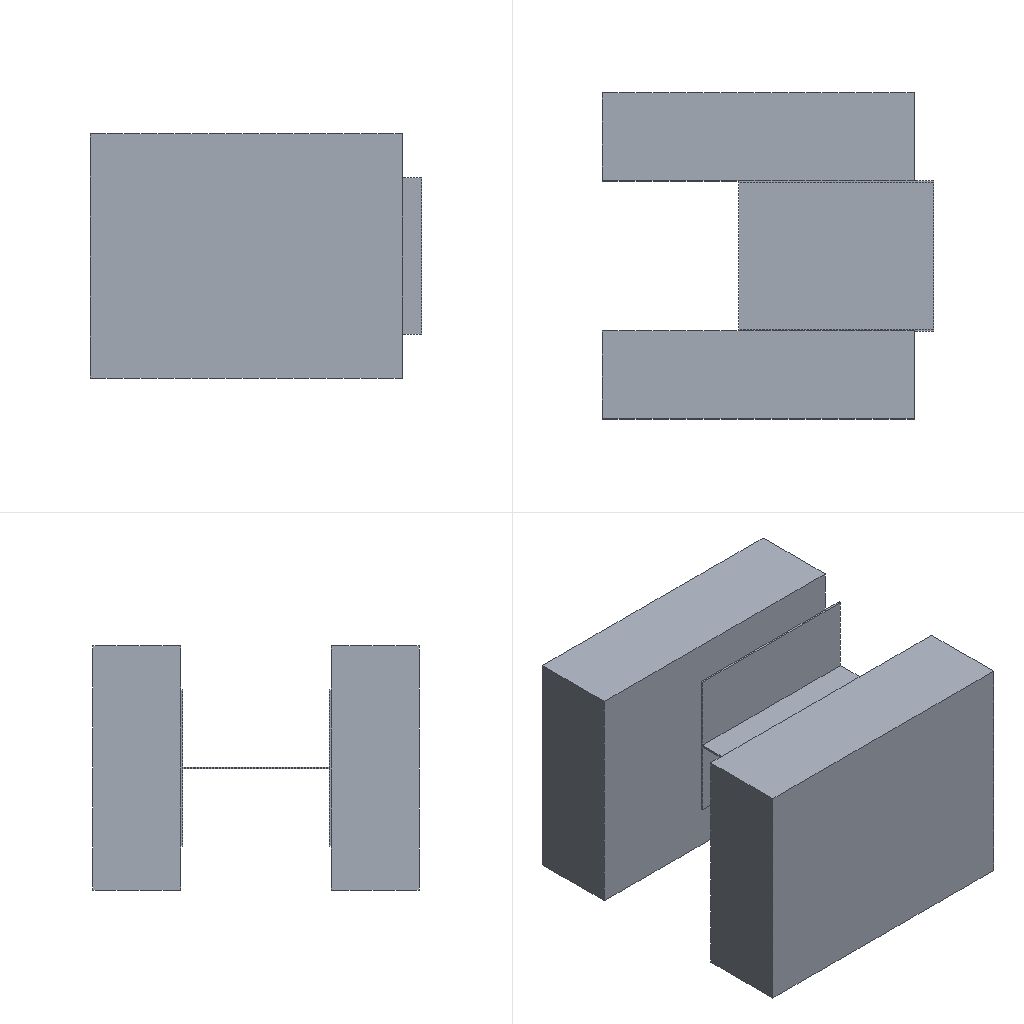Simulation study | abaqus
Set-up summary:
category,name,step,type,value,unit,region
solver,abaqus
solver,version,,,Abaqus/Explicit 2020
units,not stated in the deck,,not stated
analysis,deck,,transient,transient
load_step,Step-1,Step-1,transient
load_step,requested,,,1
mesh,nodes,,,41945
mesh,elements,,,26027
element_type,C3D8R,,solid,26027
load,load commands in deck,,count,1
bc,support commands in deck,,count,7
material,MATERIAL-1,,in results
material,STEEL,,in results
check,setup vs results,,match,"per instance, exact: element labels, types and connectivity; labels of the nodes the elements use; coordinates of those nodes at SINGLE_PRECISION in 2 of 3 instance(s)"
Abaqus input file, long lists of numbers shortened:
*Heading
** Job name: Job-1 Model name: Model-1
** Generated by: Abaqus/CAE 2020
*Preprint, echo=NO, model=NO, history=NO, contact=NO
**
** PARTS
**
*Part, name=con
*Node
      1,           0.,         -50.,         250.
      2,           0.,         -35.,         250.
** (2770 more lines like these left out)
*Element, type=C3D8R
   1,  127,  128,  135,  134,    1,    2,    9,    8
   2,  128,  129,  136,  135,    2,    3,   10,    9
** (2140 more lines like these left out)
*Nset, nset=Set-1, generate
    1,  2772,     1
*Elset, elset=Set-1, generate
    1,  2142,     1
** Section: con
*Solid Section, elset=Set-1, material=Material-1
,
*End Part
**
*Part, name=gong
*Node
      1,          -1.,          -2.,           0.
      2,          -1.,           0.,           0.
** (36399 more lines like these left out)
*Element, type=C3D8R
  1,  100,   99,    2,    1, 3018, 3084,  364,  205
  2,    4,    3,   99,  100,  206,  318, 3084, 3018
** (21741 more lines like these left out)
*Nset, nset=Set-1, generate
     1,  36401,      1
*Elset, elset=Set-1, generate
     1,  21743,      1
** Section: steel
*Solid Section, elset=Set-1, material=steel
,
*End Part
**
**
** ASSEMBLY
**
*Assembly, name=Assembly
**
*Instance, name=con-1, part=con
       -160.,           0.,           0.
*End Instance
**
*Instance, name=gong-1, part=gong
        -20.,          40.,         125.
        -20.,          40.,         125., -19.293,          40., 125.707,         180.
*End Instance
**
*Instance, name=con-2, part=con
       -160.,         244.,    -0.002505
*End Instance
**
*Node
      1,         180.,   116.979,         124.
*Nset, nset=Set-1, instance=con-1, generate
   1,  126,    1
*Nset, nset=Set-1, instance=con-2, generate
   1,  126,    1
*Elset, elset=Set-1, instance=con-1, generate
   1,  102,    1
*Elset, elset=Set-1, instance=con-2, generate
   1,  102,    1
*Nset, nset=Set-5
 1,
*Nset, nset=m_Set-2, instance=gong-1
     2,     3,     5,     9,    12,    13,    14,    15,    16,    17,    18,    19,    20,    21,    22,    23
    24,    25,    37,    38,    39,    40,    45,    46,    47,    48,    49,    50,    51,    52,    53,    54
** (498 more lines like these left out)
*Elset, elset=m_Set-2, instance=gong-1
   135,   136,   137,   138,   139,   140,   141,   142,   143,   144,   145,   146,   147,   148,   149,   150
   151,   152,   153,   154,   155,   156,   157,   158,   159,   160,   161,   162,   163,   164,   165,   166
** (358 more lines like these left out)
*Nset, nset=m_Set-4
 1,
*Nset, nset=s_Set-2, instance=con-1, generate
    1,  2772,     1
*Nset, nset=s_Set-2, instance=con-2, generate
    1,  2772,     1
*Elset, elset=s_Set-2, instance=con-1, generate
    1,  2142,     1
*Elset, elset=s_Set-2, instance=con-2, generate
    1,  2142,     1
*Elset, elset=_Surf-1_S1, internal, instance=gong-1
  3054,  3055,  3056,  3057,  3058,  3059, 10696, 10697, 10698, 10699, 10700, 10701, 10702, 10703, 10704, 10705
 10706, 10707, 10708, 10709, 10710, 10711, 10712, 10713, 10714, 10715, 10716, 10717, 10718, 10719, 10720, 10721
** (5 more lines like these left out)
*Elset, elset=_Surf-1_S4, internal, instance=gong-1
   926,   927,   928,   953,   956,   984,   988,  1001,  1012,  1685,  1688,  1689,  1691,  1693,  1695,  1696
  1698,  1701,  1702,  1703,  5655,  5656,  5657,  5683,  5686,  5712,  5716,  5729,  6424,  6426,  6427,  6429
** (1 more lines like these left out)
*Elset, elset=_Surf-1_S6, internal, instance=gong-1
   949,   950,   951,   954,  1625,  1628,  1630,  5679,  5681,  5684,  5700,  5740,  5741,  6358,  6359,  6363
  6364,  6365,  8773,  9251, 19903, 20381
*Elset, elset=_Surf-1_S3, internal, instance=gong-1
  8491,  8616,  8749,  8756,  8767,  8771,  8774,  8776,  9318,  9319,  9320,  9321,  9442,  9443,  9445,  9449
 19621, 19746, 19879, 19886, 19897, 19904, 19906, 20449, 20450, 20451, 20572, 20575, 20579, 20581
*Elset, elset=_Surf-1_S5, internal, instance=gong-1
  8495,  8613,  8615,  8762,  8775,  8777,  9452, 19625, 19743, 19745, 19892, 19901, 19905, 20570, 20573, 20583
*Elset, elset=_Surf-1_S2, internal, instance=gong-1
 133, 134
*Surface, type=ELEMENT, name=Surf-1
_Surf-1_S1, S1
_Surf-1_S4, S4
_Surf-1_S6, S6
_Surf-1_S2, S2
_Surf-1_S3, S3
_Surf-1_S5, S5
*Elset, elset=_s_Surf-2_S2, internal, instance=gong-1
 133, 134
*Elset, elset=_s_Surf-2_S4, internal, instance=gong-1
   926,   927,   928,   953,   956,   984,   988,  1001,  1012,  1685,  1688,  1689,  1691,  1693,  1695,  1696
  1698,  1701,  1702,  1703,  5655,  5656,  5657,  5683,  5686,  5712,  5716,  5729,  6424,  6426,  6427,  6429
** (1 more lines like these left out)
*Elset, elset=_s_Surf-2_S6, internal, instance=gong-1
   949,   950,   951,   954,  1625,  1628,  1630,  5679,  5681,  5684,  5700,  5740,  5741,  6358,  6359,  6363
  6364,  6365,  8773,  9251, 19903, 20381
*Elset, elset=_s_Surf-2_S1, internal, instance=gong-1
  3054,  3055,  3056,  3057,  3058,  3059, 10696, 10697, 10698, 10699, 10700, 10701, 10702, 10703, 10704, 10705
 10706, 10707, 10708, 10709, 10710, 10711, 10712, 10713, 10714, 10715, 10716, 10717, 10718, 10719, 10720, 10721
** (5 more lines like these left out)
*Elset, elset=_s_Surf-2_S3, internal, instance=gong-1
  8491,  8616,  8749,  8756,  8767,  8771,  8774,  8776,  9318,  9319,  9320,  9321,  9442,  9443,  9445,  9449
 19621, 19746, 19879, 19886, 19897, 19904, 19906, 20449, 20450, 20451, 20572, 20575, 20579, 20581
*Elset, elset=_s_Surf-2_S5, internal, instance=gong-1
  8495,  8613,  8615,  8762,  8775,  8777,  9452, 19625, 19743, 19745, 19892, 19901, 19905, 20570, 20573, 20583
*Surface, type=ELEMENT, name=s_Surf-2
_s_Surf-2_S2, S2
_s_Surf-2_S4, S4
_s_Surf-2_S6, S6
_s_Surf-2_S1, S1
_s_Surf-2_S3, S3
_s_Surf-2_S5, S5
** Constraint: Constraint-1
*Embedded Element, host elset=s_Set-2
m_Set-2
** Constraint: Constraint-2
*Coupling, constraint name=Constraint-2, ref node=m_Set-4, surface=s_Surf-2
*Kinematic
*End Assembly
*Amplitude, name=Amp-1
             0.,              0.,           0.001,              1.
**
** MATERIALS
**
*Material, name=Material-1
*Density
 2.2e-09,
*Elastic
25648., 0.25
*Concrete Damaged Plasticity
30.,    0.1,   1.16, 0.6667,   0.05
*Concrete Compression Hardening
 15.4,      0.
 16.9,  0.0002
 19.6, 0.00048
 20.1, 0.00079
  20., 0.00095
 19.6,  0.0011
 19.1, 0.00127
 18.6, 0.00143
 17.9,  0.0016
 17.2, 0.00177
 16.6, 0.00194
 15.9, 0.00211
 15.3, 0.00228
 14.7, 0.00245
 14.1, 0.00261
 13.5, 0.00278
  13., 0.00294
 12.5,  0.0031
  12., 0.00327
 11.6, 0.00343
 11.2, 0.00359
 10.8, 0.00375
 10.4, 0.00391
 10.1, 0.00406
*Concrete Tension Stiffening
 2.06,      0.
 1.92,   2e-05
 1.72,   4e-05
 1.53,   6e-05
 1.37,   8e-05
 1.24,  0.0001
 1.13, 0.00011
 1.04, 0.00013
 0.97, 0.00015
  0.9, 0.00016
 0.85, 0.00018
*Concrete Compression Damage
     0.,      0.
 0.0841,   9e-05
 0.0933,  0.0001
 0.1091, 0.00013
 0.1418,  0.0002
 0.2407, 0.00048
  0.322, 0.00079
 0.3557, 0.00095
 0.3886,  0.0011
 0.4201, 0.00127
 0.4499, 0.00143
 0.4778,  0.0016
 0.5039, 0.00177
 0.5282, 0.00194
 0.5506, 0.00211
 0.5715, 0.00228
 0.5908, 0.00245
 0.6086, 0.00261
 0.6252, 0.00278
 0.6406, 0.00294
 0.6549,  0.0031
 0.6682, 0.00327
 0.6806, 0.00343
 0.6922, 0.00359
  0.703, 0.00375
 0.7131, 0.00391
 0.7227, 0.00406
   0.74, 0.00438
 0.7554, 0.00469
 0.7691,   0.005
 0.7815, 0.00531
 0.7926, 0.00561
 0.8026, 0.00592
 0.8118, 0.00622
 0.8202, 0.00653
 0.8278, 0.00683
 0.8349, 0.00713
*Concrete Tension Damage
      0.,      0.
 0.1181,   2e-05
 0.2281,   4e-05
 0.3187,   6e-05
 0.3919,   8e-05
 0.4512,  0.0001
 0.5, 0.00011
  0.5407, 0.00013
 0.575, 0.00015
 0.6043, 0.00016
 0.6297, 0.00018
 0.7177, 0.00025
 0.7702, 0.00033
 0.8053,  0.0004
 0.8304, 0.00047
 0.8494, 0.00054
  0.8643, 0.00061
 0.8763, 0.00068
 0.8862, 0.00075
*Material, name=steel
*Density
 7.8e-09,
*Elastic
210000., 0.3
*Plastic
300.,0.
**
** INTERACTION PROPERTIES
**
*Surface Interaction, name=IntProp-1
*Friction
 0.2,
*Surface Behavior, pressure-overclosure=HARD
**
** INTERACTIONS
**
** Interaction: Int-1
*Contact, op=NEW
*Contact Inclusions, ALL EXTERIOR
*Contact Property Assignment
 ,  , IntProp-1
** ----------------------------------------------------------------
**
** STEP: Step-1
**
*Step, name=Step-1, nlgeom=YES
*Dynamic, Explicit
, 0.001
*Bulk Viscosity
0.06, 1.2
**
** BOUNDARY CONDITIONS
**
** Name: BC-1 Type: 对称/反对称/完全固定
*Boundary
Set-1, ENCASTRE
** Name: BC-2 Type: 位移/转角
*Boundary, amplitude=Amp-1
Set-5, 1, 1, -10.
Set-5, 2, 2
Set-5, 3, 3
Set-5, 4, 4
Set-5, 5, 5
Set-5, 6, 6
**
** OUTPUT REQUESTS
**
*Restart, write, number interval=1, time marks=NO
**
** FIELD OUTPUT: F-Output-1
**
*Output, field, number interval=50
*Node Output
CF, RF, U, V
*Element Output, directions=YES
DAMAGEC, DAMAGET, E, LE, MISES, PE, PEEQ, PEMAG, S, SDEG
*Contact Output
CDISP, CSTRESS
**
** HISTORY OUTPUT: H-Output-1
**
*Output, history, time interval=1e-06
*Node Output, nset=Set-5
RF1, RF2, RF3, RT, U1
*End Step
Results summary:
result,step,Step-1,completed,increments=17750 time=0.001/0.001
result,analysis,,,transient
result,last_loadstep,,,1
result,primary field,,,U
result,reaction total,,FX,53070.78,model units
result,reaction total,,FY,1929.684,model units
result,reaction total,,FZ,-6719.702,model units